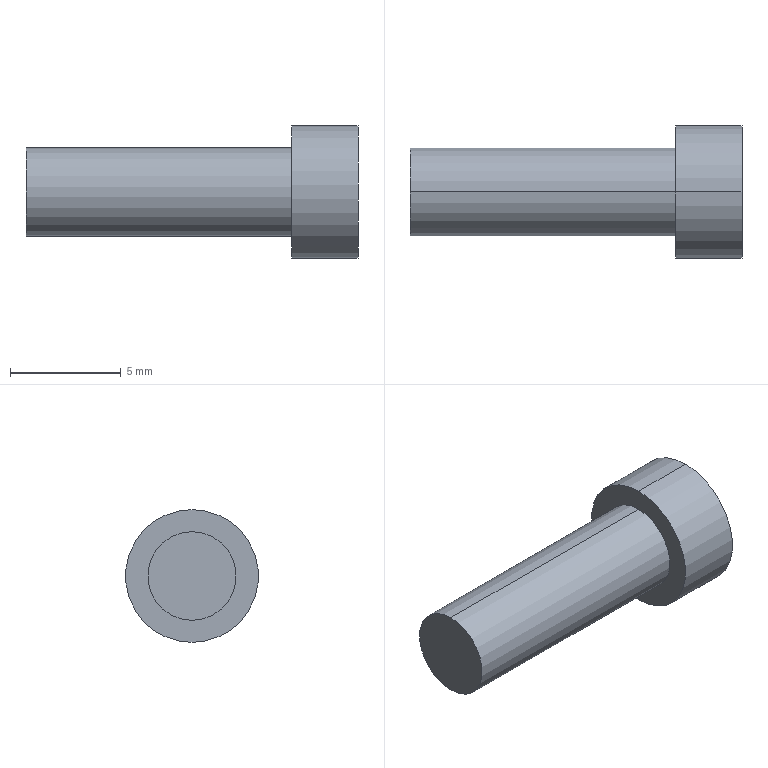Part | SolidWorks | features Revolution 1 | 1 solid | 7 faces | box 15 x 6 x 6 mm | volume 235.619 mm3 | cylinder 4 | plane 3 | commonest cylinder face diameters 4 x2 6 x2
STEP:
#1=CARTESIAN_POINT('',(1196.079,95.601,2.));
#2=VERTEX_POINT('',#1);
#3=CARTESIAN_POINT('',(1196.079,95.601,-2.));
#4=VERTEX_POINT('',#3);
#5=CARTESIAN_POINT('',(1196.079,95.601,0.));
#6=DIRECTION('',(-1.,0.,0.));
#7=DIRECTION('',(0.,0.,1.));
#8=AXIS2_PLACEMENT_3D('',#5,#6,#7);
#9=CIRCLE('',#8,2.);
#10=EDGE_CURVE('',#2,#4,#9,.T.);
#11=ORIENTED_EDGE('',*,*,#10,.T.);
#12=CARTESIAN_POINT('',(1184.079,95.601,-2.));
#13=VERTEX_POINT('',#12);
#14=CARTESIAN_POINT('',(1184.079,95.601,-2.));
#15=DIRECTION('',(-1.,0.,0.));
#16=VECTOR('',#15,1000.);
#17=LINE('',#14,#16);
#18=EDGE_CURVE('',#4,#13,#17,.T.);
#19=ORIENTED_EDGE('',*,*,#18,.T.);
#20=CARTESIAN_POINT('',(1184.079,95.601,2.));
#21=VERTEX_POINT('',#20);
#22=CARTESIAN_POINT('',(1184.079,95.601,0.));
#23=DIRECTION('',(-1.,0.,0.));
#24=DIRECTION('',(0.,0.,1.));
#25=AXIS2_PLACEMENT_3D('',#22,#23,#24);
#26=CIRCLE('',#25,2.);
#27=EDGE_CURVE('',#21,#13,#26,.T.);
#28=ORIENTED_EDGE('',*,*,#27,.F.);
#29=CARTESIAN_POINT('',(1184.079,95.601,2.));
#30=DIRECTION('',(-1.,0.,0.));
#31=VECTOR('',#30,1000.);
#32=LINE('',#29,#31);
#33=EDGE_CURVE('',#2,#21,#32,.T.);
#34=ORIENTED_EDGE('',*,*,#33,.F.);
#35=EDGE_LOOP('',(#11,#19,#28,#34));
#36=FACE_OUTER_BOUND('',#35,.T.);
#37=CARTESIAN_POINT('',(1184.079,95.601,0.));
#38=DIRECTION('',(-1.,0.,0.));
#39=DIRECTION('',(0.,0.,1.));
#40=AXIS2_PLACEMENT_3D('',#37,#38,#39);
#41=CYLINDRICAL_SURFACE('',#40,2.);
#42=ADVANCED_FACE('',(#36),#41,.T.);
#43=CARTESIAN_POINT('',(1199.079,95.601,3.));
#44=VERTEX_POINT('',#43);
#45=CARTESIAN_POINT('',(1199.079,95.601,-3.));
#46=VERTEX_POINT('',#45);
#47=CARTESIAN_POINT('',(1199.079,95.601,0.));
#48=DIRECTION('',(-1.,0.,0.));
#49=DIRECTION('',(0.,0.,1.));
#50=AXIS2_PLACEMENT_3D('',#47,#48,#49);
#51=CIRCLE('',#50,3.);
#52=EDGE_CURVE('',#44,#46,#51,.T.);
#53=ORIENTED_EDGE('',*,*,#52,.T.);
#54=CARTESIAN_POINT('',(1196.079,95.601,-3.));
#55=VERTEX_POINT('',#54);
#56=CARTESIAN_POINT('',(1184.079,95.601,-3.));
#57=DIRECTION('',(-1.,0.,0.));
#58=VECTOR('',#57,1000.);
#59=LINE('',#56,#58);
#60=EDGE_CURVE('',#46,#55,#59,.T.);
#61=ORIENTED_EDGE('',*,*,#60,.T.);
#62=CARTESIAN_POINT('',(1196.079,95.601,3.));
#63=VERTEX_POINT('',#62);
#64=CARTESIAN_POINT('',(1196.079,95.601,0.));
#65=DIRECTION('',(-1.,0.,0.));
#66=DIRECTION('',(0.,0.,1.));
#67=AXIS2_PLACEMENT_3D('',#64,#65,#66);
#68=CIRCLE('',#67,3.);
#69=EDGE_CURVE('',#63,#55,#68,.T.);
#70=ORIENTED_EDGE('',*,*,#69,.F.);
#71=CARTESIAN_POINT('',(1184.079,95.601,3.));
#72=DIRECTION('',(-1.,0.,0.));
#73=VECTOR('',#72,1000.);
#74=LINE('',#71,#73);
#75=EDGE_CURVE('',#44,#63,#74,.T.);
#76=ORIENTED_EDGE('',*,*,#75,.F.);
#77=EDGE_LOOP('',(#53,#61,#70,#76));
#78=FACE_OUTER_BOUND('',#77,.T.);
#79=CARTESIAN_POINT('',(1184.079,95.601,0.));
#80=DIRECTION('',(-1.,0.,0.));
#81=DIRECTION('',(0.,0.,1.));
#82=AXIS2_PLACEMENT_3D('',#79,#80,#81);
#83=CYLINDRICAL_SURFACE('',#82,3.);
#84=ADVANCED_FACE('',(#78),#83,.T.);
#85=ORIENTED_EDGE('',*,*,#27,.T.);
#86=CARTESIAN_POINT('',(1184.079,95.601,0.));
#87=DIRECTION('',(-1.,0.,0.));
#88=DIRECTION('',(0.,0.,1.));
#89=AXIS2_PLACEMENT_3D('',#86,#87,#88);
#90=CIRCLE('',#89,2.);
#91=EDGE_CURVE('',#13,#21,#90,.T.);
#92=ORIENTED_EDGE('',*,*,#91,.T.);
#93=EDGE_LOOP('',(#85,#92));
#94=FACE_OUTER_BOUND('',#93,.T.);
#95=CARTESIAN_POINT('',(1184.079,0.,0.));
#96=DIRECTION('',(1.,0.,0.));
#97=DIRECTION('',(0.,0.,-1.));
#98=AXIS2_PLACEMENT_3D('',#95,#96,#97);
#99=PLANE('',#98);
#100=ADVANCED_FACE('',(#94),#99,.F.);
#101=ORIENTED_EDGE('',*,*,#52,.F.);
#102=CARTESIAN_POINT('',(1199.079,95.601,0.));
#103=DIRECTION('',(-1.,0.,0.));
#104=DIRECTION('',(0.,0.,1.));
#105=AXIS2_PLACEMENT_3D('',#102,#103,#104);
#106=CIRCLE('',#105,3.);
#107=EDGE_CURVE('',#46,#44,#106,.T.);
#108=ORIENTED_EDGE('',*,*,#107,.F.);
#109=EDGE_LOOP('',(#101,#108));
#110=FACE_OUTER_BOUND('',#109,.T.);
#111=CARTESIAN_POINT('',(1199.079,0.,0.));
#112=DIRECTION('',(-1.,0.,0.));
#113=DIRECTION('',(0.,0.,1.));
#114=AXIS2_PLACEMENT_3D('',#111,#112,#113);
#115=PLANE('',#114);
#116=ADVANCED_FACE('',(#110),#115,.F.);
#117=ORIENTED_EDGE('',*,*,#60,.F.);
#118=ORIENTED_EDGE('',*,*,#107,.T.);
#119=ORIENTED_EDGE('',*,*,#75,.T.);
#120=CARTESIAN_POINT('',(1196.079,95.601,0.));
#121=DIRECTION('',(-1.,0.,0.));
#122=DIRECTION('',(0.,0.,1.));
#123=AXIS2_PLACEMENT_3D('',#120,#121,#122);
#124=CIRCLE('',#123,3.);
#125=EDGE_CURVE('',#55,#63,#124,.T.);
#126=ORIENTED_EDGE('',*,*,#125,.F.);
#127=EDGE_LOOP('',(#117,#118,#119,#126));
#128=FACE_OUTER_BOUND('',#127,.T.);
#129=CARTESIAN_POINT('',(1184.079,95.601,0.));
#130=DIRECTION('',(-1.,0.,0.));
#131=DIRECTION('',(0.,0.,1.));
#132=AXIS2_PLACEMENT_3D('',#129,#130,#131);
#133=CYLINDRICAL_SURFACE('',#132,3.);
#134=ADVANCED_FACE('',(#128),#133,.T.);
#135=ORIENTED_EDGE('',*,*,#10,.F.);
#136=CARTESIAN_POINT('',(1196.079,95.601,0.));
#137=DIRECTION('',(-1.,0.,0.));
#138=DIRECTION('',(0.,0.,1.));
#139=AXIS2_PLACEMENT_3D('',#136,#137,#138);
#140=CIRCLE('',#139,2.);
#141=EDGE_CURVE('',#4,#2,#140,.T.);
#142=ORIENTED_EDGE('',*,*,#141,.F.);
#143=EDGE_LOOP('',(#135,#142));
#144=FACE_BOUND('',#143,.T.);
#145=ORIENTED_EDGE('',*,*,#69,.T.);
#146=ORIENTED_EDGE('',*,*,#125,.T.);
#147=EDGE_LOOP('',(#145,#146));
#148=FACE_OUTER_BOUND('',#147,.T.);
#149=CARTESIAN_POINT('',(1196.079,0.,0.));
#150=DIRECTION('',(1.,0.,0.));
#151=DIRECTION('',(0.,0.,-1.));
#152=AXIS2_PLACEMENT_3D('',#149,#150,#151);
#153=PLANE('',#152);
#154=ADVANCED_FACE('',(#144,#148),#153,.F.);
#155=ORIENTED_EDGE('',*,*,#18,.F.);
#156=ORIENTED_EDGE('',*,*,#141,.T.);
#157=ORIENTED_EDGE('',*,*,#33,.T.);
#158=ORIENTED_EDGE('',*,*,#91,.F.);
#159=EDGE_LOOP('',(#155,#156,#157,#158));
#160=FACE_OUTER_BOUND('',#159,.T.);
#161=CARTESIAN_POINT('',(1184.079,95.601,0.));
#162=DIRECTION('',(-1.,0.,0.));
#163=DIRECTION('',(0.,0.,1.));
#164=AXIS2_PLACEMENT_3D('',#161,#162,#163);
#165=CYLINDRICAL_SURFACE('',#164,2.);
#166=ADVANCED_FACE('',(#160),#165,.T.);
#167=CLOSED_SHELL('',(#42,#84,#100,#116,#134,#154,#166));
#168=MANIFOLD_SOLID_BREP('',#167);
#169=CARTESIAN_POINT('',(0.,0.,0.));
#170=DIRECTION('',(0.,0.,1.));
#171=DIRECTION('',(1.,0.,0.));
#172=AXIS2_PLACEMENT_3D('',#169,#170,#171);
#173=(LENGTH_UNIT()NAMED_UNIT(*)SI_UNIT(.MILLI.,.METRE.));
#174=UNCERTAINTY_MEASURE_WITH_UNIT(LENGTH_MEASURE(0.00001),#173,'','');
#175=(NAMED_UNIT(*)PLANE_ANGLE_UNIT()SI_UNIT($,.RADIAN.));
#176=(NAMED_UNIT(*)SI_UNIT($,.STERADIAN.)SOLID_ANGLE_UNIT());
#177=(GEOMETRIC_REPRESENTATION_CONTEXT(3)GLOBAL_UNCERTAINTY_ASSIGNED_CONTEXT((#174))GLOBAL_UNIT_ASSIGNED_CONTEXT((#173,#175,#176))REPRESENTATION_CONTEXT('',''));
#178=ADVANCED_BREP_SHAPE_REPRESENTATION('',(#168,#172),#177);